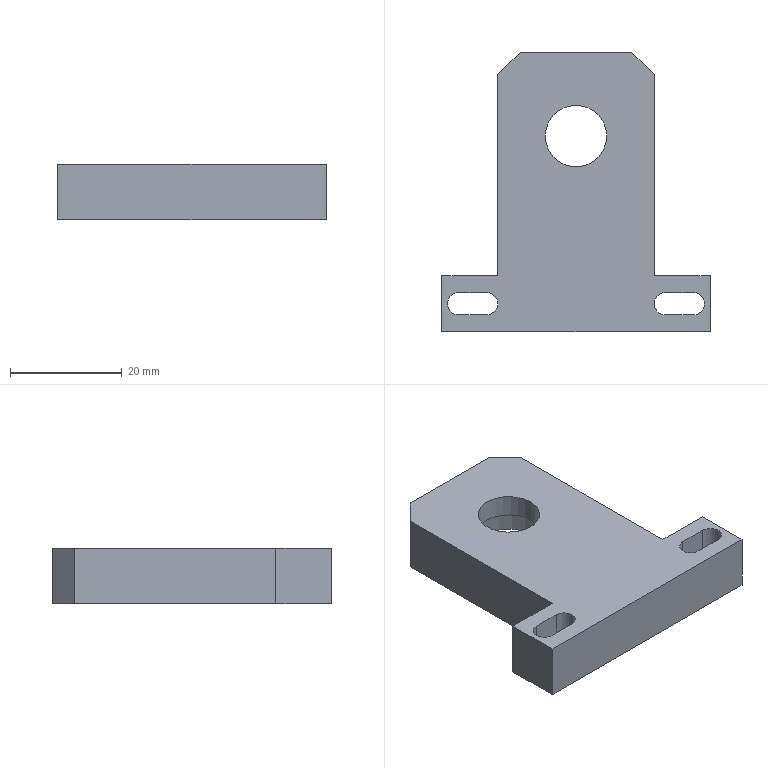Part | SolidWorks | features BaseBody 1 | 1 solid | 27 faces | box 48 x 50 x 10 mm | volume 13107 mm3 | plane 17 | cylinder 10 | commonest cylinder face diameters 4 x6 11 x2 19 x2
STEP:
#1=CARTESIAN_POINT('',(-380.5,35.,10.));
#2=VERTEX_POINT('',#1);
#3=CARTESIAN_POINT('',(-391.5,35.,10.));
#4=VERTEX_POINT('',#3);
#5=CARTESIAN_POINT('',(-386.,35.,10.));
#6=DIRECTION('',(0.,0.,-1.));
#7=DIRECTION('',(-1.,0.,0.));
#8=AXIS2_PLACEMENT_3D('',#5,#6,#7);
#9=CIRCLE('',#8,5.5);
#10=EDGE_CURVE('',#2,#4,#9,.T.);
#11=ORIENTED_EDGE('',*,*,#10,.F.);
#12=CARTESIAN_POINT('',(-380.5,35.,6.));
#13=VERTEX_POINT('',#12);
#14=CARTESIAN_POINT('',(-380.5,35.,70.029));
#15=DIRECTION('',(0.,0.,-1.));
#16=VECTOR('',#15,1000.);
#17=LINE('',#14,#16);
#18=EDGE_CURVE('',#2,#13,#17,.T.);
#19=ORIENTED_EDGE('',*,*,#18,.T.);
#20=CARTESIAN_POINT('',(-391.5,35.,6.));
#21=VERTEX_POINT('',#20);
#22=CARTESIAN_POINT('',(-386.,35.,6.));
#23=DIRECTION('',(0.,0.,1.));
#24=DIRECTION('',(-1.,0.,0.));
#25=AXIS2_PLACEMENT_3D('',#22,#23,#24);
#26=CIRCLE('',#25,5.5);
#27=EDGE_CURVE('',#21,#13,#26,.T.);
#28=ORIENTED_EDGE('',*,*,#27,.F.);
#29=CARTESIAN_POINT('',(-391.5,35.,70.029));
#30=DIRECTION('',(0.,0.,-1.));
#31=VECTOR('',#30,1000.);
#32=LINE('',#29,#31);
#33=EDGE_CURVE('',#4,#21,#32,.T.);
#34=ORIENTED_EDGE('',*,*,#33,.F.);
#35=EDGE_LOOP('',(#11,#19,#28,#34));
#36=FACE_OUTER_BOUND('',#35,.T.);
#37=CARTESIAN_POINT('',(-386.,35.,70.029));
#38=DIRECTION('',(0.,0.,-1.));
#39=DIRECTION('',(-1.,0.,0.));
#40=AXIS2_PLACEMENT_3D('',#37,#38,#39);
#41=CYLINDRICAL_SURFACE('',#40,5.5);
#42=ADVANCED_FACE('',(#36),#41,.F.);
#43=CARTESIAN_POINT('',(-409.,5.,10.));
#44=VERTEX_POINT('',#43);
#45=CARTESIAN_POINT('',(-407.,7.,10.));
#46=VERTEX_POINT('',#45);
#47=CARTESIAN_POINT('',(-407.,5.,10.));
#48=DIRECTION('',(0.,0.,-1.));
#49=DIRECTION('',(-1.,0.,0.));
#50=AXIS2_PLACEMENT_3D('',#47,#48,#49);
#51=CIRCLE('',#50,2.);
#52=EDGE_CURVE('',#44,#46,#51,.T.);
#53=ORIENTED_EDGE('',*,*,#52,.F.);
#54=CARTESIAN_POINT('',(-409.,5.,0.));
#55=VERTEX_POINT('',#54);
#56=CARTESIAN_POINT('',(-409.,5.,10.));
#57=DIRECTION('',(0.,0.,-1.));
#58=VECTOR('',#57,1000.);
#59=LINE('',#56,#58);
#60=EDGE_CURVE('',#44,#55,#59,.T.);
#61=ORIENTED_EDGE('',*,*,#60,.T.);
#62=CARTESIAN_POINT('',(-407.,7.,0.));
#63=VERTEX_POINT('',#62);
#64=CARTESIAN_POINT('',(-407.,5.,0.));
#65=DIRECTION('',(0.,0.,1.));
#66=DIRECTION('',(-1.,0.,0.));
#67=AXIS2_PLACEMENT_3D('',#64,#65,#66);
#68=CIRCLE('',#67,2.);
#69=EDGE_CURVE('',#63,#55,#68,.T.);
#70=ORIENTED_EDGE('',*,*,#69,.F.);
#71=CARTESIAN_POINT('',(-407.,7.,10.));
#72=DIRECTION('',(0.,0.,1.));
#73=VECTOR('',#72,1000.);
#74=LINE('',#71,#73);
#75=EDGE_CURVE('',#63,#46,#74,.T.);
#76=ORIENTED_EDGE('',*,*,#75,.T.);
#77=EDGE_LOOP('',(#53,#61,#70,#76));
#78=FACE_OUTER_BOUND('',#77,.T.);
#79=CARTESIAN_POINT('',(-407.,5.,10.));
#80=DIRECTION('',(0.,0.,-1.));
#81=DIRECTION('',(-1.,0.,0.));
#82=AXIS2_PLACEMENT_3D('',#79,#80,#81);
#83=CYLINDRICAL_SURFACE('',#82,2.);
#84=ADVANCED_FACE('',(#78),#83,.F.);
#85=CARTESIAN_POINT('',(-372.,5.,10.));
#86=VERTEX_POINT('',#85);
#87=CARTESIAN_POINT('',(-370.,7.,10.));
#88=VERTEX_POINT('',#87);
#89=CARTESIAN_POINT('',(-370.,5.,10.));
#90=DIRECTION('',(0.,0.,-1.));
#91=DIRECTION('',(-1.,0.,0.));
#92=AXIS2_PLACEMENT_3D('',#89,#90,#91);
#93=CIRCLE('',#92,2.);
#94=EDGE_CURVE('',#86,#88,#93,.T.);
#95=ORIENTED_EDGE('',*,*,#94,.F.);
#96=CARTESIAN_POINT('',(-372.,5.,0.));
#97=VERTEX_POINT('',#96);
#98=CARTESIAN_POINT('',(-372.,5.,10.));
#99=DIRECTION('',(0.,0.,-1.));
#100=VECTOR('',#99,1000.);
#101=LINE('',#98,#100);
#102=EDGE_CURVE('',#86,#97,#101,.T.);
#103=ORIENTED_EDGE('',*,*,#102,.T.);
#104=CARTESIAN_POINT('',(-370.,7.,0.));
#105=VERTEX_POINT('',#104);
#106=CARTESIAN_POINT('',(-370.,5.,0.));
#107=DIRECTION('',(0.,0.,1.));
#108=DIRECTION('',(-1.,0.,0.));
#109=AXIS2_PLACEMENT_3D('',#106,#107,#108);
#110=CIRCLE('',#109,2.);
#111=EDGE_CURVE('',#105,#97,#110,.T.);
#112=ORIENTED_EDGE('',*,*,#111,.F.);
#113=CARTESIAN_POINT('',(-370.,7.,10.));
#114=DIRECTION('',(0.,0.,1.));
#115=VECTOR('',#114,1000.);
#116=LINE('',#113,#115);
#117=EDGE_CURVE('',#105,#88,#116,.T.);
#118=ORIENTED_EDGE('',*,*,#117,.T.);
#119=EDGE_LOOP('',(#95,#103,#112,#118));
#120=FACE_OUTER_BOUND('',#119,.T.);
#121=CARTESIAN_POINT('',(-370.,5.,10.));
#122=DIRECTION('',(0.,0.,-1.));
#123=DIRECTION('',(-1.,0.,0.));
#124=AXIS2_PLACEMENT_3D('',#121,#122,#123);
#125=CYLINDRICAL_SURFACE('',#124,2.);
#126=ADVANCED_FACE('',(#120),#125,.F.);
#127=CARTESIAN_POINT('',(-376.5,35.,6.));
#128=VERTEX_POINT('',#127);
#129=CARTESIAN_POINT('',(-395.5,35.,6.));
#130=VERTEX_POINT('',#129);
#131=CARTESIAN_POINT('',(-386.,35.,6.));
#132=DIRECTION('',(0.,0.,-1.));
#133=DIRECTION('',(-1.,0.,0.));
#134=AXIS2_PLACEMENT_3D('',#131,#132,#133);
#135=CIRCLE('',#134,9.5);
#136=EDGE_CURVE('',#128,#130,#135,.T.);
#137=ORIENTED_EDGE('',*,*,#136,.F.);
#138=CARTESIAN_POINT('',(-376.5,35.,0.));
#139=VERTEX_POINT('',#138);
#140=CARTESIAN_POINT('',(-376.5,35.,3.));
#141=DIRECTION('',(0.,0.,-1.));
#142=VECTOR('',#141,1000.);
#143=LINE('',#140,#142);
#144=EDGE_CURVE('',#128,#139,#143,.T.);
#145=ORIENTED_EDGE('',*,*,#144,.T.);
#146=CARTESIAN_POINT('',(-395.5,35.,0.));
#147=VERTEX_POINT('',#146);
#148=CARTESIAN_POINT('',(-386.,35.,0.));
#149=DIRECTION('',(0.,0.,-1.));
#150=DIRECTION('',(-1.,0.,0.));
#151=AXIS2_PLACEMENT_3D('',#148,#149,#150);
#152=CIRCLE('',#151,9.5);
#153=EDGE_CURVE('',#139,#147,#152,.T.);
#154=ORIENTED_EDGE('',*,*,#153,.T.);
#155=CARTESIAN_POINT('',(-395.5,35.,3.));
#156=DIRECTION('',(0.,0.,-1.));
#157=VECTOR('',#156,1000.);
#158=LINE('',#155,#157);
#159=EDGE_CURVE('',#130,#147,#158,.T.);
#160=ORIENTED_EDGE('',*,*,#159,.F.);
#161=EDGE_LOOP('',(#137,#145,#154,#160));
#162=FACE_OUTER_BOUND('',#161,.T.);
#163=CARTESIAN_POINT('',(-386.,35.,3.));
#164=DIRECTION('',(0.,0.,-1.));
#165=DIRECTION('',(-1.,0.,0.));
#166=AXIS2_PLACEMENT_3D('',#163,#164,#165);
#167=CYLINDRICAL_SURFACE('',#166,9.5);
#168=ADVANCED_FACE('',(#162),#167,.F.);
#169=CARTESIAN_POINT('',(-386.,35.,10.));
#170=DIRECTION('',(0.,0.,-1.));
#171=DIRECTION('',(-1.,0.,0.));
#172=AXIS2_PLACEMENT_3D('',#169,#170,#171);
#173=CIRCLE('',#172,5.5);
#174=EDGE_CURVE('',#4,#2,#173,.T.);
#175=ORIENTED_EDGE('',*,*,#174,.T.);
#176=ORIENTED_EDGE('',*,*,#10,.T.);
#177=EDGE_LOOP('',(#175,#176));
#178=FACE_BOUND('',#177,.T.);
#179=CARTESIAN_POINT('',(-407.,3.,10.));
#180=VERTEX_POINT('',#179);
#181=CARTESIAN_POINT('',(-407.,5.,10.));
#182=DIRECTION('',(0.,0.,-1.));
#183=DIRECTION('',(-1.,0.,0.));
#184=AXIS2_PLACEMENT_3D('',#181,#182,#183);
#185=CIRCLE('',#184,2.);
#186=EDGE_CURVE('',#180,#44,#185,.T.);
#187=ORIENTED_EDGE('',*,*,#186,.T.);
#188=ORIENTED_EDGE('',*,*,#52,.T.);
#189=CARTESIAN_POINT('',(-402.,7.,10.));
#190=VERTEX_POINT('',#189);
#191=CARTESIAN_POINT('',(-386.,7.,10.));
#192=DIRECTION('',(1.,0.,0.));
#193=VECTOR('',#192,1000.);
#194=LINE('',#191,#193);
#195=EDGE_CURVE('',#46,#190,#194,.T.);
#196=ORIENTED_EDGE('',*,*,#195,.T.);
#197=CARTESIAN_POINT('',(-402.,3.,10.));
#198=VERTEX_POINT('',#197);
#199=CARTESIAN_POINT('',(-402.,5.,10.));
#200=DIRECTION('',(0.,0.,-1.));
#201=DIRECTION('',(-1.,0.,0.));
#202=AXIS2_PLACEMENT_3D('',#199,#200,#201);
#203=CIRCLE('',#202,2.);
#204=EDGE_CURVE('',#190,#198,#203,.T.);
#205=ORIENTED_EDGE('',*,*,#204,.T.);
#206=CARTESIAN_POINT('',(-386.,3.,10.));
#207=DIRECTION('',(-1.,0.,0.));
#208=VECTOR('',#207,1000.);
#209=LINE('',#206,#208);
#210=EDGE_CURVE('',#198,#180,#209,.T.);
#211=ORIENTED_EDGE('',*,*,#210,.T.);
#212=EDGE_LOOP('',(#187,#188,#196,#205,#211));
#213=FACE_BOUND('',#212,.T.);
#214=CARTESIAN_POINT('',(-370.,3.,10.));
#215=VERTEX_POINT('',#214);
#216=CARTESIAN_POINT('',(-370.,5.,10.));
#217=DIRECTION('',(0.,0.,-1.));
#218=DIRECTION('',(-1.,0.,0.));
#219=AXIS2_PLACEMENT_3D('',#216,#217,#218);
#220=CIRCLE('',#219,2.);
#221=EDGE_CURVE('',#215,#86,#220,.T.);
#222=ORIENTED_EDGE('',*,*,#221,.T.);
#223=ORIENTED_EDGE('',*,*,#94,.T.);
#224=CARTESIAN_POINT('',(-365.,7.,10.));
#225=VERTEX_POINT('',#224);
#226=CARTESIAN_POINT('',(-386.,7.,10.));
#227=DIRECTION('',(1.,0.,0.));
#228=VECTOR('',#227,1000.);
#229=LINE('',#226,#228);
#230=EDGE_CURVE('',#88,#225,#229,.T.);
#231=ORIENTED_EDGE('',*,*,#230,.T.);
#232=CARTESIAN_POINT('',(-365.,3.,10.));
#233=VERTEX_POINT('',#232);
#234=CARTESIAN_POINT('',(-365.,5.,10.));
#235=DIRECTION('',(0.,0.,-1.));
#236=DIRECTION('',(-1.,0.,0.));
#237=AXIS2_PLACEMENT_3D('',#234,#235,#236);
#238=CIRCLE('',#237,2.);
#239=EDGE_CURVE('',#225,#233,#238,.T.);
#240=ORIENTED_EDGE('',*,*,#239,.T.);
#241=CARTESIAN_POINT('',(-386.,3.,10.));
#242=DIRECTION('',(-1.,0.,0.));
#243=VECTOR('',#242,1000.);
#244=LINE('',#241,#243);
#245=EDGE_CURVE('',#233,#215,#244,.T.);
#246=ORIENTED_EDGE('',*,*,#245,.T.);
#247=EDGE_LOOP('',(#222,#223,#231,#240,#246));
#248=FACE_BOUND('',#247,.T.);
#249=CARTESIAN_POINT('',(-362.,10.,10.));
#250=VERTEX_POINT('',#249);
#251=CARTESIAN_POINT('',(-372.,10.,10.));
#252=VERTEX_POINT('',#251);
#253=CARTESIAN_POINT('',(-386.,10.,10.));
#254=DIRECTION('',(-1.,0.,0.));
#255=VECTOR('',#254,1000.);
#256=LINE('',#253,#255);
#257=EDGE_CURVE('',#250,#252,#256,.T.);
#258=ORIENTED_EDGE('',*,*,#257,.T.);
#259=CARTESIAN_POINT('',(-372.,46.,10.));
#260=VERTEX_POINT('',#259);
#261=CARTESIAN_POINT('',(-372.,25.,10.));
#262=DIRECTION('',(0.,1.,0.));
#263=VECTOR('',#262,1000.);
#264=LINE('',#261,#263);
#265=EDGE_CURVE('',#252,#260,#264,.T.);
#266=ORIENTED_EDGE('',*,*,#265,.T.);
#267=CARTESIAN_POINT('',(-376.,50.,10.));
#268=VERTEX_POINT('',#267);
#269=CARTESIAN_POINT('',(-372.,46.,10.));
#270=DIRECTION('',(-0.7071,0.7071,0.));
#271=VECTOR('',#270,1000.);
#272=LINE('',#269,#271);
#273=EDGE_CURVE('',#260,#268,#272,.T.);
#274=ORIENTED_EDGE('',*,*,#273,.T.);
#275=CARTESIAN_POINT('',(-396.,50.,10.));
#276=VERTEX_POINT('',#275);
#277=CARTESIAN_POINT('',(-386.,50.,10.));
#278=DIRECTION('',(-1.,0.,0.));
#279=VECTOR('',#278,1000.);
#280=LINE('',#277,#279);
#281=EDGE_CURVE('',#268,#276,#280,.T.);
#282=ORIENTED_EDGE('',*,*,#281,.T.);
#283=CARTESIAN_POINT('',(-400.,46.,10.));
#284=VERTEX_POINT('',#283);
#285=CARTESIAN_POINT('',(-396.,50.,10.));
#286=DIRECTION('',(-0.7071,-0.7071,0.));
#287=VECTOR('',#286,1000.);
#288=LINE('',#285,#287);
#289=EDGE_CURVE('',#276,#284,#288,.T.);
#290=ORIENTED_EDGE('',*,*,#289,.T.);
#291=CARTESIAN_POINT('',(-400.,10.,10.));
#292=VERTEX_POINT('',#291);
#293=CARTESIAN_POINT('',(-400.,25.,10.));
#294=DIRECTION('',(0.,-1.,0.));
#295=VECTOR('',#294,1000.);
#296=LINE('',#293,#295);
#297=EDGE_CURVE('',#284,#292,#296,.T.);
#298=ORIENTED_EDGE('',*,*,#297,.T.);
#299=CARTESIAN_POINT('',(-410.,10.,10.));
#300=VERTEX_POINT('',#299);
#301=CARTESIAN_POINT('',(-386.,10.,10.));
#302=DIRECTION('',(-1.,0.,0.));
#303=VECTOR('',#302,1000.);
#304=LINE('',#301,#303);
#305=EDGE_CURVE('',#292,#300,#304,.T.);
#306=ORIENTED_EDGE('',*,*,#305,.T.);
#307=CARTESIAN_POINT('',(-410.,0.,10.));
#308=VERTEX_POINT('',#307);
#309=CARTESIAN_POINT('',(-410.,25.,10.));
#310=DIRECTION('',(0.,-1.,0.));
#311=VECTOR('',#310,1000.);
#312=LINE('',#309,#311);
#313=EDGE_CURVE('',#300,#308,#312,.T.);
#314=ORIENTED_EDGE('',*,*,#313,.T.);
#315=CARTESIAN_POINT('',(-362.,0.,10.));
#316=VERTEX_POINT('',#315);
#317=CARTESIAN_POINT('',(-386.,0.,10.));
#318=DIRECTION('',(1.,0.,0.));
#319=VECTOR('',#318,1000.);
#320=LINE('',#317,#319);
#321=EDGE_CURVE('',#308,#316,#320,.T.);
#322=ORIENTED_EDGE('',*,*,#321,.T.);
#323=CARTESIAN_POINT('',(-362.,25.,10.));
#324=DIRECTION('',(0.,1.,0.));
#325=VECTOR('',#324,1000.);
#326=LINE('',#323,#325);
#327=EDGE_CURVE('',#316,#250,#326,.T.);
#328=ORIENTED_EDGE('',*,*,#327,.T.);
#329=EDGE_LOOP('',(#258,#266,#274,#282,#290,#298,#306,#314,#322,#328));
#330=FACE_OUTER_BOUND('',#329,.T.);
#331=CARTESIAN_POINT('',(-386.,25.,10.));
#332=DIRECTION('',(0.,0.,1.));
#333=DIRECTION('',(1.,0.,0.));
#334=AXIS2_PLACEMENT_3D('',#331,#332,#333);
#335=PLANE('',#334);
#336=ADVANCED_FACE('',(#178,#213,#248,#330),#335,.T.);
#337=ORIENTED_EDGE('',*,*,#18,.F.);
#338=ORIENTED_EDGE('',*,*,#174,.F.);
#339=ORIENTED_EDGE('',*,*,#33,.T.);
#340=CARTESIAN_POINT('',(-386.,35.,6.));
#341=DIRECTION('',(0.,0.,1.));
#342=DIRECTION('',(-1.,0.,0.));
#343=AXIS2_PLACEMENT_3D('',#340,#341,#342);
#344=CIRCLE('',#343,5.5);
#345=EDGE_CURVE('',#13,#21,#344,.T.);
#346=ORIENTED_EDGE('',*,*,#345,.F.);
#347=EDGE_LOOP('',(#337,#338,#339,#346));
#348=FACE_OUTER_BOUND('',#347,.T.);
#349=CARTESIAN_POINT('',(-386.,35.,70.029));
#350=DIRECTION('',(0.,0.,-1.));
#351=DIRECTION('',(-1.,0.,0.));
#352=AXIS2_PLACEMENT_3D('',#349,#350,#351);
#353=CYLINDRICAL_SURFACE('',#352,5.5);
#354=ADVANCED_FACE('',(#348),#353,.F.);
#355=CARTESIAN_POINT('',(-402.,7.,0.));
#356=VERTEX_POINT('',#355);
#357=CARTESIAN_POINT('',(-402.,7.,10.));
#358=DIRECTION('',(0.,0.,-1.));
#359=VECTOR('',#358,1000.);
#360=LINE('',#357,#359);
#361=EDGE_CURVE('',#190,#356,#360,.T.);
#362=ORIENTED_EDGE('',*,*,#361,.F.);
#363=ORIENTED_EDGE('',*,*,#195,.F.);
#364=ORIENTED_EDGE('',*,*,#75,.F.);
#365=CARTESIAN_POINT('',(-402.,7.,0.));
#366=DIRECTION('',(-1.,0.,0.));
#367=VECTOR('',#366,1000.);
#368=LINE('',#365,#367);
#369=EDGE_CURVE('',#356,#63,#368,.T.);
#370=ORIENTED_EDGE('',*,*,#369,.F.);
#371=EDGE_LOOP('',(#362,#363,#364,#370));
#372=FACE_OUTER_BOUND('',#371,.T.);
#373=CARTESIAN_POINT('',(-402.,7.,10.));
#374=DIRECTION('',(0.,1.,0.));
#375=DIRECTION('',(0.,0.,1.));
#376=AXIS2_PLACEMENT_3D('',#373,#374,#375);
#377=PLANE('',#376);
#378=ADVANCED_FACE('',(#372),#377,.F.);
#379=ORIENTED_EDGE('',*,*,#60,.F.);
#380=ORIENTED_EDGE('',*,*,#186,.F.);
#381=CARTESIAN_POINT('',(-407.,3.,0.));
#382=VERTEX_POINT('',#381);
#383=CARTESIAN_POINT('',(-407.,3.,10.));
#384=DIRECTION('',(0.,0.,1.));
#385=VECTOR('',#384,1000.);
#386=LINE('',#383,#385);
#387=EDGE_CURVE('',#382,#180,#386,.T.);
#388=ORIENTED_EDGE('',*,*,#387,.F.);
#389=CARTESIAN_POINT('',(-407.,5.,0.));
#390=DIRECTION('',(0.,0.,1.));
#391=DIRECTION('',(-1.,0.,0.));
#392=AXIS2_PLACEMENT_3D('',#389,#390,#391);
#393=CIRCLE('',#392,2.);
#394=EDGE_CURVE('',#55,#382,#393,.T.);
#395=ORIENTED_EDGE('',*,*,#394,.F.);
#396=EDGE_LOOP('',(#379,#380,#388,#395));
#397=FACE_OUTER_BOUND('',#396,.T.);
#398=CARTESIAN_POINT('',(-407.,5.,10.));
#399=DIRECTION('',(0.,0.,-1.));
#400=DIRECTION('',(-1.,0.,0.));
#401=AXIS2_PLACEMENT_3D('',#398,#399,#400);
#402=CYLINDRICAL_SURFACE('',#401,2.);
#403=ADVANCED_FACE('',(#397),#402,.F.);
#404=ORIENTED_EDGE('',*,*,#387,.T.);
#405=ORIENTED_EDGE('',*,*,#210,.F.);
#406=CARTESIAN_POINT('',(-402.,3.,0.));
#407=VERTEX_POINT('',#406);
#408=CARTESIAN_POINT('',(-402.,3.,10.));
#409=DIRECTION('',(0.,0.,1.));
#410=VECTOR('',#409,1000.);
#411=LINE('',#408,#410);
#412=EDGE_CURVE('',#407,#198,#411,.T.);
#413=ORIENTED_EDGE('',*,*,#412,.F.);
#414=CARTESIAN_POINT('',(-407.,3.,0.));
#415=DIRECTION('',(1.,0.,0.));
#416=VECTOR('',#415,1000.);
#417=LINE('',#414,#416);
#418=EDGE_CURVE('',#382,#407,#417,.T.);
#419=ORIENTED_EDGE('',*,*,#418,.F.);
#420=EDGE_LOOP('',(#404,#405,#413,#419));
#421=FACE_OUTER_BOUND('',#420,.T.);
#422=CARTESIAN_POINT('',(-407.,3.,10.));
#423=DIRECTION('',(0.,-1.,0.));
#424=DIRECTION('',(0.,0.,-1.));
#425=AXIS2_PLACEMENT_3D('',#422,#423,#424);
#426=PLANE('',#425);
#427=ADVANCED_FACE('',(#421),#426,.F.);
#428=ORIENTED_EDGE('',*,*,#412,.T.);
#429=ORIENTED_EDGE('',*,*,#204,.F.);
#430=ORIENTED_EDGE('',*,*,#361,.T.);
#431=CARTESIAN_POINT('',(-402.,5.,0.));
#432=DIRECTION('',(0.,0.,1.));
#433=DIRECTION('',(-1.,0.,0.));
#434=AXIS2_PLACEMENT_3D('',#431,#432,#433);
#435=CIRCLE('',#434,2.);
#436=EDGE_CURVE('',#407,#356,#435,.T.);
#437=ORIENTED_EDGE('',*,*,#436,.F.);
#438=EDGE_LOOP('',(#428,#429,#430,#437));
#439=FACE_OUTER_BOUND('',#438,.T.);
#440=CARTESIAN_POINT('',(-402.,5.,10.));
#441=DIRECTION('',(0.,0.,-1.));
#442=DIRECTION('',(-1.,0.,0.));
#443=AXIS2_PLACEMENT_3D('',#440,#441,#442);
#444=CYLINDRICAL_SURFACE('',#443,2.);
#445=ADVANCED_FACE('',(#439),#444,.F.);
#446=CARTESIAN_POINT('',(-365.,7.,0.));
#447=VERTEX_POINT('',#446);
#448=CARTESIAN_POINT('',(-365.,7.,10.));
#449=DIRECTION('',(0.,0.,-1.));
#450=VECTOR('',#449,1000.);
#451=LINE('',#448,#450);
#452=EDGE_CURVE('',#225,#447,#451,.T.);
#453=ORIENTED_EDGE('',*,*,#452,.F.);
#454=ORIENTED_EDGE('',*,*,#230,.F.);
#455=ORIENTED_EDGE('',*,*,#117,.F.);
#456=CARTESIAN_POINT('',(-365.,7.,0.));
#457=DIRECTION('',(-1.,0.,0.));
#458=VECTOR('',#457,1000.);
#459=LINE('',#456,#458);
#460=EDGE_CURVE('',#447,#105,#459,.T.);
#461=ORIENTED_EDGE('',*,*,#460,.F.);
#462=EDGE_LOOP('',(#453,#454,#455,#461));
#463=FACE_OUTER_BOUND('',#462,.T.);
#464=CARTESIAN_POINT('',(-365.,7.,10.));
#465=DIRECTION('',(0.,1.,0.));
#466=DIRECTION('',(0.,0.,1.));
#467=AXIS2_PLACEMENT_3D('',#464,#465,#466);
#468=PLANE('',#467);
#469=ADVANCED_FACE('',(#463),#468,.F.);
#470=ORIENTED_EDGE('',*,*,#102,.F.);
#471=ORIENTED_EDGE('',*,*,#221,.F.);
#472=CARTESIAN_POINT('',(-370.,3.,0.));
#473=VERTEX_POINT('',#472);
#474=CARTESIAN_POINT('',(-370.,3.,10.));
#475=DIRECTION('',(0.,0.,1.));
#476=VECTOR('',#475,1000.);
#477=LINE('',#474,#476);
#478=EDGE_CURVE('',#473,#215,#477,.T.);
#479=ORIENTED_EDGE('',*,*,#478,.F.);
#480=CARTESIAN_POINT('',(-370.,5.,0.));
#481=DIRECTION('',(0.,0.,1.));
#482=DIRECTION('',(-1.,0.,0.));
#483=AXIS2_PLACEMENT_3D('',#480,#481,#482);
#484=CIRCLE('',#483,2.);
#485=EDGE_CURVE('',#97,#473,#484,.T.);
#486=ORIENTED_EDGE('',*,*,#485,.F.);
#487=EDGE_LOOP('',(#470,#471,#479,#486));
#488=FACE_OUTER_BOUND('',#487,.T.);
#489=CARTESIAN_POINT('',(-370.,5.,10.));
#490=DIRECTION('',(0.,0.,-1.));
#491=DIRECTION('',(-1.,0.,0.));
#492=AXIS2_PLACEMENT_3D('',#489,#490,#491);
#493=CYLINDRICAL_SURFACE('',#492,2.);
#494=ADVANCED_FACE('',(#488),#493,.F.);
#495=ORIENTED_EDGE('',*,*,#478,.T.);
#496=ORIENTED_EDGE('',*,*,#245,.F.);
#497=CARTESIAN_POINT('',(-365.,3.,0.));
#498=VERTEX_POINT('',#497);
#499=CARTESIAN_POINT('',(-365.,3.,10.));
#500=DIRECTION('',(0.,0.,1.));
#501=VECTOR('',#500,1000.);
#502=LINE('',#499,#501);
#503=EDGE_CURVE('',#498,#233,#502,.T.);
#504=ORIENTED_EDGE('',*,*,#503,.F.);
#505=CARTESIAN_POINT('',(-370.,3.,0.));
#506=DIRECTION('',(1.,0.,0.));
#507=VECTOR('',#506,1000.);
#508=LINE('',#505,#507);
#509=EDGE_CURVE('',#473,#498,#508,.T.);
#510=ORIENTED_EDGE('',*,*,#509,.F.);
#511=EDGE_LOOP('',(#495,#496,#504,#510));
#512=FACE_OUTER_BOUND('',#511,.T.);
#513=CARTESIAN_POINT('',(-370.,3.,10.));
#514=DIRECTION('',(0.,-1.,0.));
#515=DIRECTION('',(0.,0.,-1.));
#516=AXIS2_PLACEMENT_3D('',#513,#514,#515);
#517=PLANE('',#516);
#518=ADVANCED_FACE('',(#512),#517,.F.);
#519=ORIENTED_EDGE('',*,*,#503,.T.);
#520=ORIENTED_EDGE('',*,*,#239,.F.);
#521=ORIENTED_EDGE('',*,*,#452,.T.);
#522=CARTESIAN_POINT('',(-365.,5.,0.));
#523=DIRECTION('',(0.,0.,1.));
#524=DIRECTION('',(-1.,0.,0.));
#525=AXIS2_PLACEMENT_3D('',#522,#523,#524);
#526=CIRCLE('',#525,2.);
#527=EDGE_CURVE('',#498,#447,#526,.T.);
#528=ORIENTED_EDGE('',*,*,#527,.F.);
#529=EDGE_LOOP('',(#519,#520,#521,#528));
#530=FACE_OUTER_BOUND('',#529,.T.);
#531=CARTESIAN_POINT('',(-365.,5.,10.));
#532=DIRECTION('',(0.,0.,-1.));
#533=DIRECTION('',(-1.,0.,0.));
#534=AXIS2_PLACEMENT_3D('',#531,#532,#533);
#535=CYLINDRICAL_SURFACE('',#534,2.);
#536=ADVANCED_FACE('',(#530),#535,.F.);
#537=ORIENTED_EDGE('',*,*,#265,.F.);
#538=CARTESIAN_POINT('',(-372.,10.,0.));
#539=VERTEX_POINT('',#538);
#540=CARTESIAN_POINT('',(-372.,10.,10.));
#541=DIRECTION('',(0.,0.,1.));
#542=VECTOR('',#541,1000.);
#543=LINE('',#540,#542);
#544=EDGE_CURVE('',#539,#252,#543,.T.);
#545=ORIENTED_EDGE('',*,*,#544,.F.);
#546=CARTESIAN_POINT('',(-372.,46.,0.));
#547=VERTEX_POINT('',#546);
#548=CARTESIAN_POINT('',(-372.,50.,0.));
#549=DIRECTION('',(0.,-1.,0.));
#550=VECTOR('',#549,1000.);
#551=LINE('',#548,#550);
#552=EDGE_CURVE('',#547,#539,#551,.T.);
#553=ORIENTED_EDGE('',*,*,#552,.F.);
#554=CARTESIAN_POINT('',(-372.,46.,10.));
#555=DIRECTION('',(0.,0.,-1.));
#556=VECTOR('',#555,1000.);
#557=LINE('',#554,#556);
#558=EDGE_CURVE('',#260,#547,#557,.T.);
#559=ORIENTED_EDGE('',*,*,#558,.F.);
#560=EDGE_LOOP('',(#537,#545,#553,#559));
#561=FACE_OUTER_BOUND('',#560,.T.);
#562=CARTESIAN_POINT('',(-372.,50.,10.));
#563=DIRECTION('',(-1.,0.,0.));
#564=DIRECTION('',(0.,0.,1.));
#565=AXIS2_PLACEMENT_3D('',#562,#563,#564);
#566=PLANE('',#565);
#567=ADVANCED_FACE('',(#561),#566,.F.);
#568=ORIENTED_EDGE('',*,*,#544,.T.);
#569=ORIENTED_EDGE('',*,*,#257,.F.);
#570=CARTESIAN_POINT('',(-362.,10.,0.));
#571=VERTEX_POINT('',#570);
#572=CARTESIAN_POINT('',(-362.,10.,10.));
#573=DIRECTION('',(0.,0.,1.));
#574=VECTOR('',#573,1000.);
#575=LINE('',#572,#574);
#576=EDGE_CURVE('',#571,#250,#575,.T.);
#577=ORIENTED_EDGE('',*,*,#576,.F.);
#578=CARTESIAN_POINT('',(-372.,10.,0.));
#579=DIRECTION('',(1.,0.,0.));
#580=VECTOR('',#579,1000.);
#581=LINE('',#578,#580);
#582=EDGE_CURVE('',#539,#571,#581,.T.);
#583=ORIENTED_EDGE('',*,*,#582,.F.);
#584=EDGE_LOOP('',(#568,#569,#577,#583));
#585=FACE_OUTER_BOUND('',#584,.T.);
#586=CARTESIAN_POINT('',(-372.,10.,10.));
#587=DIRECTION('',(0.,-1.,0.));
#588=DIRECTION('',(0.,0.,-1.));
#589=AXIS2_PLACEMENT_3D('',#586,#587,#588);
#590=PLANE('',#589);
#591=ADVANCED_FACE('',(#585),#590,.F.);
#592=CARTESIAN_POINT('',(-362.,0.,0.));
#593=VERTEX_POINT('',#592);
#594=CARTESIAN_POINT('',(-362.,0.,0.));
#595=DIRECTION('',(0.,0.,-1.));
#596=VECTOR('',#595,1000.);
#597=LINE('',#594,#596);
#598=EDGE_CURVE('',#316,#593,#597,.T.);
#599=ORIENTED_EDGE('',*,*,#598,.T.);
#600=CARTESIAN_POINT('',(-362.,50.,0.));
#601=DIRECTION('',(0.,1.,0.));
#602=VECTOR('',#601,1000.);
#603=LINE('',#600,#602);
#604=EDGE_CURVE('',#593,#571,#603,.T.);
#605=ORIENTED_EDGE('',*,*,#604,.T.);
#606=ORIENTED_EDGE('',*,*,#576,.T.);
#607=ORIENTED_EDGE('',*,*,#327,.F.);
#608=EDGE_LOOP('',(#599,#605,#606,#607));
#609=FACE_OUTER_BOUND('',#608,.T.);
#610=CARTESIAN_POINT('',(-362.,50.,0.));
#611=DIRECTION('',(1.,0.,0.));
#612=DIRECTION('',(0.,0.,-1.));
#613=AXIS2_PLACEMENT_3D('',#610,#611,#612);
#614=PLANE('',#613);
#615=ADVANCED_FACE('',(#609),#614,.T.);
#616=CARTESIAN_POINT('',(-410.,0.,0.));
#617=VERTEX_POINT('',#616);
#618=CARTESIAN_POINT('',(-362.,0.,0.));
#619=DIRECTION('',(1.,0.,0.));
#620=VECTOR('',#619,1000.);
#621=LINE('',#618,#620);
#622=EDGE_CURVE('',#617,#593,#621,.T.);
#623=ORIENTED_EDGE('',*,*,#622,.T.);
#624=ORIENTED_EDGE('',*,*,#598,.F.);
#625=ORIENTED_EDGE('',*,*,#321,.F.);
#626=CARTESIAN_POINT('',(-410.,0.,0.));
#627=DIRECTION('',(0.,0.,-1.));
#628=VECTOR('',#627,1000.);
#629=LINE('',#626,#628);
#630=EDGE_CURVE('',#308,#617,#629,.T.);
#631=ORIENTED_EDGE('',*,*,#630,.T.);
#632=EDGE_LOOP('',(#623,#624,#625,#631));
#633=FACE_OUTER_BOUND('',#632,.T.);
#634=CARTESIAN_POINT('',(-362.,0.,0.));
#635=DIRECTION('',(0.,-1.,0.));
#636=DIRECTION('',(0.,0.,-1.));
#637=AXIS2_PLACEMENT_3D('',#634,#635,#636);
#638=PLANE('',#637);
#639=ADVANCED_FACE('',(#633),#638,.T.);
#640=ORIENTED_EDGE('',*,*,#630,.F.);
#641=ORIENTED_EDGE('',*,*,#313,.F.);
#642=CARTESIAN_POINT('',(-410.,10.,0.));
#643=VERTEX_POINT('',#642);
#644=CARTESIAN_POINT('',(-410.,10.,0.));
#645=DIRECTION('',(0.,0.,-1.));
#646=VECTOR('',#645,1000.);
#647=LINE('',#644,#646);
#648=EDGE_CURVE('',#300,#643,#647,.T.);
#649=ORIENTED_EDGE('',*,*,#648,.T.);
#650=CARTESIAN_POINT('',(-410.,0.,0.));
#651=DIRECTION('',(0.,-1.,0.));
#652=VECTOR('',#651,1000.);
#653=LINE('',#650,#652);
#654=EDGE_CURVE('',#643,#617,#653,.T.);
#655=ORIENTED_EDGE('',*,*,#654,.T.);
#656=EDGE_LOOP('',(#640,#641,#649,#655));
#657=FACE_OUTER_BOUND('',#656,.T.);
#658=CARTESIAN_POINT('',(-410.,0.,0.));
#659=DIRECTION('',(-1.,0.,0.));
#660=DIRECTION('',(0.,0.,1.));
#661=AXIS2_PLACEMENT_3D('',#658,#659,#660);
#662=PLANE('',#661);
#663=ADVANCED_FACE('',(#657),#662,.T.);
#664=ORIENTED_EDGE('',*,*,#648,.F.);
#665=ORIENTED_EDGE('',*,*,#305,.F.);
#666=CARTESIAN_POINT('',(-400.,10.,0.));
#667=VERTEX_POINT('',#666);
#668=CARTESIAN_POINT('',(-400.,10.,10.));
#669=DIRECTION('',(0.,0.,1.));
#670=VECTOR('',#669,1000.);
#671=LINE('',#668,#670);
#672=EDGE_CURVE('',#667,#292,#671,.T.);
#673=ORIENTED_EDGE('',*,*,#672,.F.);
#674=CARTESIAN_POINT('',(-410.,10.,0.));
#675=DIRECTION('',(1.,0.,0.));
#676=VECTOR('',#675,1000.);
#677=LINE('',#674,#676);
#678=EDGE_CURVE('',#643,#667,#677,.T.);
#679=ORIENTED_EDGE('',*,*,#678,.F.);
#680=EDGE_LOOP('',(#664,#665,#673,#679));
#681=FACE_OUTER_BOUND('',#680,.T.);
#682=CARTESIAN_POINT('',(-410.,10.,10.));
#683=DIRECTION('',(0.,-1.,0.));
#684=DIRECTION('',(0.,0.,-1.));
#685=AXIS2_PLACEMENT_3D('',#682,#683,#684);
#686=PLANE('',#685);
#687=ADVANCED_FACE('',(#681),#686,.F.);
#688=CARTESIAN_POINT('',(-400.,46.,0.));
#689=VERTEX_POINT('',#688);
#690=CARTESIAN_POINT('',(-400.,10.,0.));
#691=DIRECTION('',(0.,1.,0.));
#692=VECTOR('',#691,1000.);
#693=LINE('',#690,#692);
#694=EDGE_CURVE('',#667,#689,#693,.T.);
#695=ORIENTED_EDGE('',*,*,#694,.F.);
#696=ORIENTED_EDGE('',*,*,#672,.T.);
#697=ORIENTED_EDGE('',*,*,#297,.F.);
#698=CARTESIAN_POINT('',(-400.,46.,10.));
#699=DIRECTION('',(0.,0.,1.));
#700=VECTOR('',#699,1000.);
#701=LINE('',#698,#700);
#702=EDGE_CURVE('',#689,#284,#701,.T.);
#703=ORIENTED_EDGE('',*,*,#702,.F.);
#704=EDGE_LOOP('',(#695,#696,#697,#703));
#705=FACE_OUTER_BOUND('',#704,.T.);
#706=CARTESIAN_POINT('',(-400.,10.,10.));
#707=DIRECTION('',(1.,0.,0.));
#708=DIRECTION('',(0.,0.,-1.));
#709=AXIS2_PLACEMENT_3D('',#706,#707,#708);
#710=PLANE('',#709);
#711=ADVANCED_FACE('',(#705),#710,.F.);
#712=CARTESIAN_POINT('',(-396.,50.,0.));
#713=VERTEX_POINT('',#712);
#714=CARTESIAN_POINT('',(-398.,48.,0.));
#715=DIRECTION('',(-0.7071,-0.7071,0.));
#716=VECTOR('',#715,1000.);
#717=LINE('',#714,#716);
#718=EDGE_CURVE('',#713,#689,#717,.T.);
#719=ORIENTED_EDGE('',*,*,#718,.T.);
#720=ORIENTED_EDGE('',*,*,#702,.T.);
#721=ORIENTED_EDGE('',*,*,#289,.F.);
#722=CARTESIAN_POINT('',(-396.,50.,5.));
#723=DIRECTION('',(0.,0.,-1.));
#724=VECTOR('',#723,1000.);
#725=LINE('',#722,#724);
#726=EDGE_CURVE('',#276,#713,#725,.T.);
#727=ORIENTED_EDGE('',*,*,#726,.T.);
#728=EDGE_LOOP('',(#719,#720,#721,#727));
#729=FACE_OUTER_BOUND('',#728,.T.);
#730=CARTESIAN_POINT('',(-398.,48.,5.));
#731=DIRECTION('',(-0.7071,0.7071,0.));
#732=DIRECTION('',(-0.7071,-0.7071,0.));
#733=AXIS2_PLACEMENT_3D('',#730,#731,#732);
#734=PLANE('',#733);
#735=ADVANCED_FACE('',(#729),#734,.T.);
#736=ORIENTED_EDGE('',*,*,#726,.F.);
#737=ORIENTED_EDGE('',*,*,#281,.F.);
#738=CARTESIAN_POINT('',(-376.,50.,0.));
#739=VERTEX_POINT('',#738);
#740=CARTESIAN_POINT('',(-376.,50.,0.));
#741=DIRECTION('',(0.,0.,-1.));
#742=VECTOR('',#741,1000.);
#743=LINE('',#740,#742);
#744=EDGE_CURVE('',#268,#739,#743,.T.);
#745=ORIENTED_EDGE('',*,*,#744,.T.);
#746=CARTESIAN_POINT('',(-410.,50.,0.));
#747=DIRECTION('',(-1.,0.,0.));
#748=VECTOR('',#747,1000.);
#749=LINE('',#746,#748);
#750=EDGE_CURVE('',#739,#713,#749,.T.);
#751=ORIENTED_EDGE('',*,*,#750,.T.);
#752=EDGE_LOOP('',(#736,#737,#745,#751));
#753=FACE_OUTER_BOUND('',#752,.T.);
#754=CARTESIAN_POINT('',(-410.,50.,0.));
#755=DIRECTION('',(0.,1.,0.));
#756=DIRECTION('',(0.,0.,1.));
#757=AXIS2_PLACEMENT_3D('',#754,#755,#756);
#758=PLANE('',#757);
#759=ADVANCED_FACE('',(#753),#758,.T.);
#760=ORIENTED_EDGE('',*,*,#273,.F.);
#761=ORIENTED_EDGE('',*,*,#558,.T.);
#762=CARTESIAN_POINT('',(-374.,48.,0.));
#763=DIRECTION('',(-0.7071,0.7071,0.));
#764=VECTOR('',#763,1000.);
#765=LINE('',#762,#764);
#766=EDGE_CURVE('',#547,#739,#765,.T.);
#767=ORIENTED_EDGE('',*,*,#766,.T.);
#768=ORIENTED_EDGE('',*,*,#744,.F.);
#769=EDGE_LOOP('',(#760,#761,#767,#768));
#770=FACE_OUTER_BOUND('',#769,.T.);
#771=CARTESIAN_POINT('',(-374.,48.,5.));
#772=DIRECTION('',(0.7071,0.7071,0.));
#773=DIRECTION('',(-0.7071,0.7071,0.));
#774=AXIS2_PLACEMENT_3D('',#771,#772,#773);
#775=PLANE('',#774);
#776=ADVANCED_FACE('',(#770),#775,.T.);
#777=ORIENTED_EDGE('',*,*,#27,.T.);
#778=ORIENTED_EDGE('',*,*,#345,.T.);
#779=EDGE_LOOP('',(#777,#778));
#780=FACE_BOUND('',#779,.T.);
#781=CARTESIAN_POINT('',(-386.,35.,6.));
#782=DIRECTION('',(0.,0.,-1.));
#783=DIRECTION('',(-1.,0.,0.));
#784=AXIS2_PLACEMENT_3D('',#781,#782,#783);
#785=CIRCLE('',#784,9.5);
#786=EDGE_CURVE('',#130,#128,#785,.T.);
#787=ORIENTED_EDGE('',*,*,#786,.T.);
#788=ORIENTED_EDGE('',*,*,#136,.T.);
#789=EDGE_LOOP('',(#787,#788));
#790=FACE_OUTER_BOUND('',#789,.T.);
#791=CARTESIAN_POINT('',(-386.,35.,6.));
#792=DIRECTION('',(0.,0.,-1.));
#793=DIRECTION('',(-1.,0.,0.));
#794=AXIS2_PLACEMENT_3D('',#791,#792,#793);
#795=PLANE('',#794);
#796=ADVANCED_FACE('',(#780,#790),#795,.T.);
#797=CARTESIAN_POINT('',(-386.,35.,0.));
#798=DIRECTION('',(0.,0.,-1.));
#799=DIRECTION('',(-1.,0.,0.));
#800=AXIS2_PLACEMENT_3D('',#797,#798,#799);
#801=CIRCLE('',#800,9.5);
#802=EDGE_CURVE('',#147,#139,#801,.T.);
#803=ORIENTED_EDGE('',*,*,#802,.F.);
#804=ORIENTED_EDGE('',*,*,#153,.F.);
#805=EDGE_LOOP('',(#803,#804));
#806=FACE_BOUND('',#805,.T.);
#807=ORIENTED_EDGE('',*,*,#369,.T.);
#808=ORIENTED_EDGE('',*,*,#69,.T.);
#809=ORIENTED_EDGE('',*,*,#394,.T.);
#810=ORIENTED_EDGE('',*,*,#418,.T.);
#811=ORIENTED_EDGE('',*,*,#436,.T.);
#812=EDGE_LOOP('',(#807,#808,#809,#810,#811));
#813=FACE_BOUND('',#812,.T.);
#814=ORIENTED_EDGE('',*,*,#460,.T.);
#815=ORIENTED_EDGE('',*,*,#111,.T.);
#816=ORIENTED_EDGE('',*,*,#485,.T.);
#817=ORIENTED_EDGE('',*,*,#509,.T.);
#818=ORIENTED_EDGE('',*,*,#527,.T.);
#819=EDGE_LOOP('',(#814,#815,#816,#817,#818));
#820=FACE_BOUND('',#819,.T.);
#821=ORIENTED_EDGE('',*,*,#552,.T.);
#822=ORIENTED_EDGE('',*,*,#582,.T.);
#823=ORIENTED_EDGE('',*,*,#604,.F.);
#824=ORIENTED_EDGE('',*,*,#622,.F.);
#825=ORIENTED_EDGE('',*,*,#654,.F.);
#826=ORIENTED_EDGE('',*,*,#678,.T.);
#827=ORIENTED_EDGE('',*,*,#694,.T.);
#828=ORIENTED_EDGE('',*,*,#718,.F.);
#829=ORIENTED_EDGE('',*,*,#750,.F.);
#830=ORIENTED_EDGE('',*,*,#766,.F.);
#831=EDGE_LOOP('',(#821,#822,#823,#824,#825,#826,#827,#828,#829,#830));
#832=FACE_OUTER_BOUND('',#831,.T.);
#833=CARTESIAN_POINT('',(-386.,25.,0.));
#834=DIRECTION('',(0.,0.,1.));
#835=DIRECTION('',(1.,0.,0.));
#836=AXIS2_PLACEMENT_3D('',#833,#834,#835);
#837=PLANE('',#836);
#838=ADVANCED_FACE('',(#806,#813,#820,#832),#837,.F.);
#839=ORIENTED_EDGE('',*,*,#144,.F.);
#840=ORIENTED_EDGE('',*,*,#786,.F.);
#841=ORIENTED_EDGE('',*,*,#159,.T.);
#842=ORIENTED_EDGE('',*,*,#802,.T.);
#843=EDGE_LOOP('',(#839,#840,#841,#842));
#844=FACE_OUTER_BOUND('',#843,.T.);
#845=CARTESIAN_POINT('',(-386.,35.,3.));
#846=DIRECTION('',(0.,0.,-1.));
#847=DIRECTION('',(-1.,0.,0.));
#848=AXIS2_PLACEMENT_3D('',#845,#846,#847);
#849=CYLINDRICAL_SURFACE('',#848,9.5);
#850=ADVANCED_FACE('',(#844),#849,.F.);
#851=CLOSED_SHELL('',(#42,#84,#126,#168,#336,#354,#378,#403,#427,#445,#469,#494,#518,#536,#567,#591,#615,#639,#663,#687,#711,#735,#759,#776,#796,#838,#850));
#852=MANIFOLD_SOLID_BREP('',#851);
#853=CARTESIAN_POINT('',(0.,0.,0.));
#854=DIRECTION('',(0.,0.,1.));
#855=DIRECTION('',(1.,0.,0.));
#856=AXIS2_PLACEMENT_3D('',#853,#854,#855);
#857=(LENGTH_UNIT()NAMED_UNIT(*)SI_UNIT(.MILLI.,.METRE.));
#858=UNCERTAINTY_MEASURE_WITH_UNIT(LENGTH_MEASURE(0.00001),#857,'','');
#859=(NAMED_UNIT(*)PLANE_ANGLE_UNIT()SI_UNIT($,.RADIAN.));
#860=(NAMED_UNIT(*)SI_UNIT($,.STERADIAN.)SOLID_ANGLE_UNIT());
#861=(GEOMETRIC_REPRESENTATION_CONTEXT(3)GLOBAL_UNCERTAINTY_ASSIGNED_CONTEXT((#858))GLOBAL_UNIT_ASSIGNED_CONTEXT((#857,#859,#860))REPRESENTATION_CONTEXT('',''));
#862=ADVANCED_BREP_SHAPE_REPRESENTATION('',(#852,#856),#861);